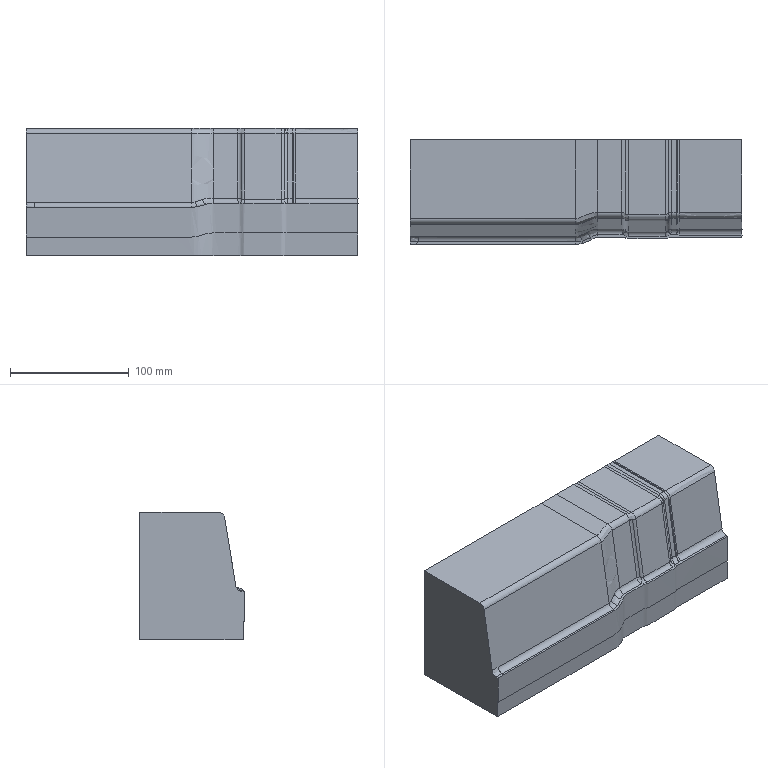Part | NX | features solid 2 | 1 solid | 73 faces | box 280 x 88.161 x 107.138 mm | volume 2308062 mm3 | spline 30 | plane 20 | cylinder 20 | cone 3 | commonest cylinder face diameters 10 x9 8 x5 12 x3 20 x2 14 x1